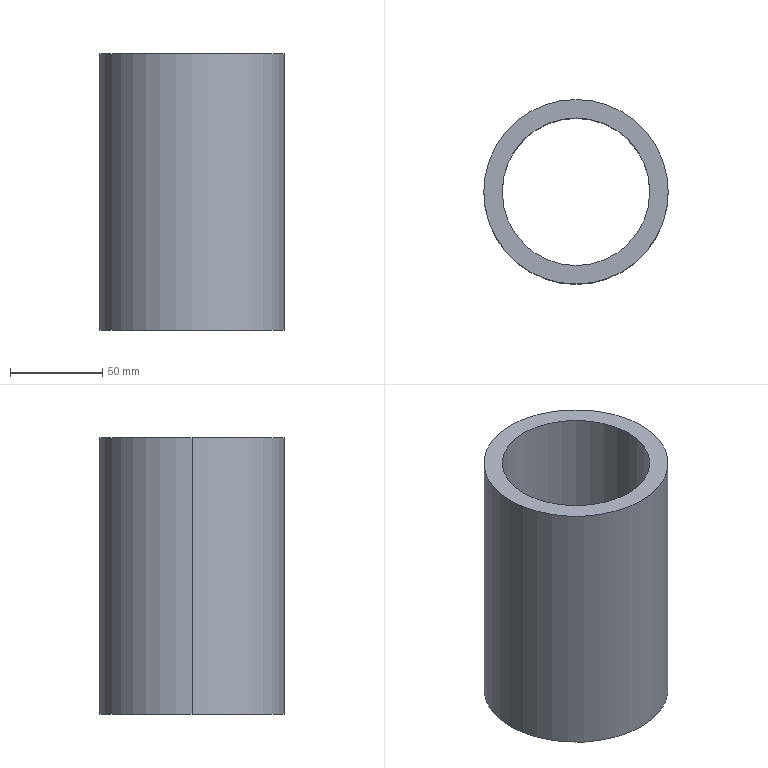Part | SolidWorks | features Extrusion 1 | 1 solid | 6 faces | box 100 x 100 x 150 mm | volume 424115 mm3 | cylinder 4 | plane 2 | commonest cylinder face diameters 80 x2 100 x2
STEP:
#1=CARTESIAN_POINT('',(-40.,0.,150.));
#2=VERTEX_POINT('',#1);
#3=CARTESIAN_POINT('',(40.,0.,150.));
#4=VERTEX_POINT('',#3);
#5=CARTESIAN_POINT('',(0.,0.,150.));
#6=DIRECTION('',(0.,0.,1.));
#7=DIRECTION('',(1.,0.,0.));
#8=AXIS2_PLACEMENT_3D('',#5,#6,#7);
#9=CIRCLE('',#8,40.);
#10=EDGE_CURVE('',#2,#4,#9,.T.);
#11=ORIENTED_EDGE('',*,*,#10,.T.);
#12=CARTESIAN_POINT('',(40.,0.,0.));
#13=VERTEX_POINT('',#12);
#14=CARTESIAN_POINT('',(40.,0.,150.));
#15=DIRECTION('',(0.,0.,-1.));
#16=VECTOR('',#15,1000.);
#17=LINE('',#14,#16);
#18=EDGE_CURVE('',#4,#13,#17,.T.);
#19=ORIENTED_EDGE('',*,*,#18,.T.);
#20=CARTESIAN_POINT('',(-40.,0.,0.));
#21=VERTEX_POINT('',#20);
#22=CARTESIAN_POINT('',(0.,0.,0.));
#23=DIRECTION('',(0.,0.,1.));
#24=DIRECTION('',(1.,0.,0.));
#25=AXIS2_PLACEMENT_3D('',#22,#23,#24);
#26=CIRCLE('',#25,40.);
#27=EDGE_CURVE('',#21,#13,#26,.T.);
#28=ORIENTED_EDGE('',*,*,#27,.F.);
#29=CARTESIAN_POINT('',(-40.,0.,150.));
#30=DIRECTION('',(0.,0.,-1.));
#31=VECTOR('',#30,1000.);
#32=LINE('',#29,#31);
#33=EDGE_CURVE('',#2,#21,#32,.T.);
#34=ORIENTED_EDGE('',*,*,#33,.F.);
#35=EDGE_LOOP('',(#11,#19,#28,#34));
#36=FACE_OUTER_BOUND('',#35,.T.);
#37=CARTESIAN_POINT('',(0.,0.,150.));
#38=DIRECTION('',(0.,0.,-1.));
#39=DIRECTION('',(-1.,0.,0.));
#40=AXIS2_PLACEMENT_3D('',#37,#38,#39);
#41=CYLINDRICAL_SURFACE('',#40,40.);
#42=ADVANCED_FACE('',(#36),#41,.F.);
#43=CARTESIAN_POINT('',(50.,0.,150.));
#44=VERTEX_POINT('',#43);
#45=CARTESIAN_POINT('',(-50.,0.,150.));
#46=VERTEX_POINT('',#45);
#47=CARTESIAN_POINT('',(0.,0.,150.));
#48=DIRECTION('',(0.,0.,1.));
#49=DIRECTION('',(1.,0.,0.));
#50=AXIS2_PLACEMENT_3D('',#47,#48,#49);
#51=CIRCLE('',#50,50.);
#52=EDGE_CURVE('',#44,#46,#51,.T.);
#53=ORIENTED_EDGE('',*,*,#52,.F.);
#54=CARTESIAN_POINT('',(50.,0.,0.));
#55=VERTEX_POINT('',#54);
#56=CARTESIAN_POINT('',(50.,0.,150.));
#57=DIRECTION('',(0.,0.,-1.));
#58=VECTOR('',#57,1000.);
#59=LINE('',#56,#58);
#60=EDGE_CURVE('',#44,#55,#59,.T.);
#61=ORIENTED_EDGE('',*,*,#60,.T.);
#62=CARTESIAN_POINT('',(-50.,0.,0.));
#63=VERTEX_POINT('',#62);
#64=CARTESIAN_POINT('',(0.,0.,0.));
#65=DIRECTION('',(0.,0.,1.));
#66=DIRECTION('',(1.,0.,0.));
#67=AXIS2_PLACEMENT_3D('',#64,#65,#66);
#68=CIRCLE('',#67,50.);
#69=EDGE_CURVE('',#55,#63,#68,.T.);
#70=ORIENTED_EDGE('',*,*,#69,.T.);
#71=CARTESIAN_POINT('',(-50.,0.,150.));
#72=DIRECTION('',(0.,0.,-1.));
#73=VECTOR('',#72,1000.);
#74=LINE('',#71,#73);
#75=EDGE_CURVE('',#46,#63,#74,.T.);
#76=ORIENTED_EDGE('',*,*,#75,.F.);
#77=EDGE_LOOP('',(#53,#61,#70,#76));
#78=FACE_OUTER_BOUND('',#77,.T.);
#79=CARTESIAN_POINT('',(0.,0.,150.));
#80=DIRECTION('',(0.,0.,-1.));
#81=DIRECTION('',(-1.,0.,0.));
#82=AXIS2_PLACEMENT_3D('',#79,#80,#81);
#83=CYLINDRICAL_SURFACE('',#82,50.);
#84=ADVANCED_FACE('',(#78),#83,.T.);
#85=CARTESIAN_POINT('',(0.,0.,150.));
#86=DIRECTION('',(0.,0.,1.));
#87=DIRECTION('',(1.,0.,0.));
#88=AXIS2_PLACEMENT_3D('',#85,#86,#87);
#89=CIRCLE('',#88,50.);
#90=EDGE_CURVE('',#46,#44,#89,.T.);
#91=ORIENTED_EDGE('',*,*,#90,.T.);
#92=ORIENTED_EDGE('',*,*,#52,.T.);
#93=EDGE_LOOP('',(#91,#92));
#94=FACE_OUTER_BOUND('',#93,.T.);
#95=ORIENTED_EDGE('',*,*,#10,.F.);
#96=CARTESIAN_POINT('',(0.,0.,150.));
#97=DIRECTION('',(0.,0.,1.));
#98=DIRECTION('',(1.,0.,0.));
#99=AXIS2_PLACEMENT_3D('',#96,#97,#98);
#100=CIRCLE('',#99,40.);
#101=EDGE_CURVE('',#4,#2,#100,.T.);
#102=ORIENTED_EDGE('',*,*,#101,.F.);
#103=EDGE_LOOP('',(#95,#102));
#104=FACE_BOUND('',#103,.T.);
#105=CARTESIAN_POINT('',(0.,0.,150.));
#106=DIRECTION('',(0.,0.,1.));
#107=DIRECTION('',(1.,0.,0.));
#108=AXIS2_PLACEMENT_3D('',#105,#106,#107);
#109=PLANE('',#108);
#110=ADVANCED_FACE('',(#94,#104),#109,.T.);
#111=CARTESIAN_POINT('',(0.,0.,0.));
#112=DIRECTION('',(0.,0.,1.));
#113=DIRECTION('',(1.,0.,0.));
#114=AXIS2_PLACEMENT_3D('',#111,#112,#113);
#115=CIRCLE('',#114,50.);
#116=EDGE_CURVE('',#63,#55,#115,.T.);
#117=ORIENTED_EDGE('',*,*,#116,.F.);
#118=ORIENTED_EDGE('',*,*,#69,.F.);
#119=EDGE_LOOP('',(#117,#118));
#120=FACE_OUTER_BOUND('',#119,.T.);
#121=ORIENTED_EDGE('',*,*,#27,.T.);
#122=CARTESIAN_POINT('',(0.,0.,0.));
#123=DIRECTION('',(0.,0.,1.));
#124=DIRECTION('',(1.,0.,0.));
#125=AXIS2_PLACEMENT_3D('',#122,#123,#124);
#126=CIRCLE('',#125,40.);
#127=EDGE_CURVE('',#13,#21,#126,.T.);
#128=ORIENTED_EDGE('',*,*,#127,.T.);
#129=EDGE_LOOP('',(#121,#128));
#130=FACE_BOUND('',#129,.T.);
#131=CARTESIAN_POINT('',(0.,0.,0.));
#132=DIRECTION('',(0.,0.,1.));
#133=DIRECTION('',(1.,0.,0.));
#134=AXIS2_PLACEMENT_3D('',#131,#132,#133);
#135=PLANE('',#134);
#136=ADVANCED_FACE('',(#120,#130),#135,.F.);
#137=ORIENTED_EDGE('',*,*,#60,.F.);
#138=ORIENTED_EDGE('',*,*,#90,.F.);
#139=ORIENTED_EDGE('',*,*,#75,.T.);
#140=ORIENTED_EDGE('',*,*,#116,.T.);
#141=EDGE_LOOP('',(#137,#138,#139,#140));
#142=FACE_OUTER_BOUND('',#141,.T.);
#143=CARTESIAN_POINT('',(0.,0.,150.));
#144=DIRECTION('',(0.,0.,-1.));
#145=DIRECTION('',(-1.,0.,0.));
#146=AXIS2_PLACEMENT_3D('',#143,#144,#145);
#147=CYLINDRICAL_SURFACE('',#146,50.);
#148=ADVANCED_FACE('',(#142),#147,.T.);
#149=ORIENTED_EDGE('',*,*,#18,.F.);
#150=ORIENTED_EDGE('',*,*,#101,.T.);
#151=ORIENTED_EDGE('',*,*,#33,.T.);
#152=ORIENTED_EDGE('',*,*,#127,.F.);
#153=EDGE_LOOP('',(#149,#150,#151,#152));
#154=FACE_OUTER_BOUND('',#153,.T.);
#155=CARTESIAN_POINT('',(0.,0.,150.));
#156=DIRECTION('',(0.,0.,-1.));
#157=DIRECTION('',(-1.,0.,0.));
#158=AXIS2_PLACEMENT_3D('',#155,#156,#157);
#159=CYLINDRICAL_SURFACE('',#158,40.);
#160=ADVANCED_FACE('',(#154),#159,.F.);
#161=CLOSED_SHELL('',(#42,#84,#110,#136,#148,#160));
#162=MANIFOLD_SOLID_BREP('',#161);
#163=CARTESIAN_POINT('',(0.,0.,0.));
#164=DIRECTION('',(0.,0.,1.));
#165=DIRECTION('',(1.,0.,0.));
#166=AXIS2_PLACEMENT_3D('',#163,#164,#165);
#167=(LENGTH_UNIT()NAMED_UNIT(*)SI_UNIT(.MILLI.,.METRE.));
#168=UNCERTAINTY_MEASURE_WITH_UNIT(LENGTH_MEASURE(0.00001),#167,'','');
#169=(NAMED_UNIT(*)PLANE_ANGLE_UNIT()SI_UNIT($,.RADIAN.));
#170=(NAMED_UNIT(*)SI_UNIT($,.STERADIAN.)SOLID_ANGLE_UNIT());
#171=(GEOMETRIC_REPRESENTATION_CONTEXT(3)GLOBAL_UNCERTAINTY_ASSIGNED_CONTEXT((#168))GLOBAL_UNIT_ASSIGNED_CONTEXT((#167,#169,#170))REPRESENTATION_CONTEXT('',''));
#172=ADVANCED_BREP_SHAPE_REPRESENTATION('',(#162,#166),#171);